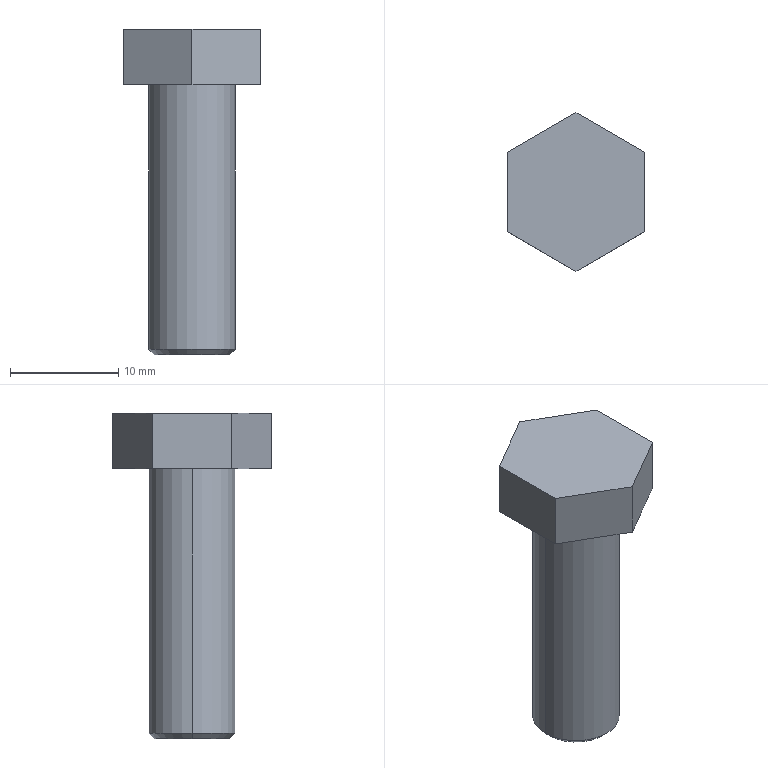Part | STEP file | Bulong M8_2.5F | 1 solid | 13 faces | box 12.73 x 14.699 x 30.15 mm | volume 1976 mm3 | plane 9 | cone 2 | cylinder 2 | commonest cylinder face diameters 8 x2
STEP:
#1=CARTESIAN_POINT('',(0.,0.,0.));
#2=DIRECTION('',(0.,0.,1.));
#3=DIRECTION('',(1.,0.,0.));
#4=AXIS2_PLACEMENT_3D('',#1,#2,#3);
#5=CARTESIAN_POINT('',(-3.5,0.,-25.));
#6=VERTEX_POINT('',#5);
#7=CARTESIAN_POINT('',(3.5,0.,-25.));
#8=VERTEX_POINT('',#7);
#9=CARTESIAN_POINT('',(0.,0.,-25.));
#10=DIRECTION('',(0.,0.,-1.));
#11=DIRECTION('',(-1.,0.,0.));
#12=AXIS2_PLACEMENT_3D('',#9,#10,#11);
#13=CIRCLE('',#12,3.5);
#14=CARTESIAN_POINT('',(0.,0.,-25.));
#15=DIRECTION('',(0.,0.,1.));
#16=DIRECTION('',(1.,0.,0.));
#17=AXIS2_PLACEMENT_3D('',#14,#15,#16);
#18=CONICAL_SURFACE('',#17,3.5,0.7854);
#19=CARTESIAN_POINT('',(3.142,0.));
#20=DIRECTION('',(-1.,0.));
#21=VECTOR('',#20,1.);
#22=LINE('',#19,#21);
#23=(GEOMETRIC_REPRESENTATION_CONTEXT(2)PARAMETRIC_REPRESENTATION_CONTEXT()REPRESENTATION_CONTEXT('',''));
#24=DEFINITIONAL_REPRESENTATION('',(#22),#23);
#25=PCURVE('',#18,#24);
#26=CARTESIAN_POINT('',(0.,0.,-25.));
#27=DIRECTION('',(0.,0.,-1.));
#28=DIRECTION('',(-1.,0.,0.));
#29=AXIS2_PLACEMENT_3D('',#26,#27,#28);
#30=PLANE('',#29);
#31=CARTESIAN_POINT('',(0.,0.));
#32=DIRECTION('',(1.,0.));
#33=AXIS2_PLACEMENT_2D('',#31,#32);
#34=CIRCLE('',#33,3.5);
#35=(GEOMETRIC_REPRESENTATION_CONTEXT(2)PARAMETRIC_REPRESENTATION_CONTEXT()REPRESENTATION_CONTEXT('',''));
#36=DEFINITIONAL_REPRESENTATION('',(#34),#35);
#37=PCURVE('',#30,#36);
#38=SURFACE_CURVE('',#13,(#25,#37),.PCURVE_S1.);
#39=EDGE_CURVE('',#6,#8,#38,.T.);
#40=ORIENTED_EDGE('',*,*,#39,.F.);
#41=CARTESIAN_POINT('',(-4.,0.,-24.5));
#42=VERTEX_POINT('',#41);
#43=CARTESIAN_POINT('',(-3.5,0.,-25.));
#44=DIRECTION('',(-0.7071,0.,0.7071));
#45=VECTOR('',#44,1.);
#46=LINE('',#43,#45);
#47=CARTESIAN_POINT('',(3.142,0.));
#48=DIRECTION('',(0.,1.));
#49=VECTOR('',#48,1.);
#50=LINE('',#47,#49);
#51=(GEOMETRIC_REPRESENTATION_CONTEXT(2)PARAMETRIC_REPRESENTATION_CONTEXT()REPRESENTATION_CONTEXT('',''));
#52=DEFINITIONAL_REPRESENTATION('',(#50),#51);
#53=PCURVE('',#18,#52);
#54=CARTESIAN_POINT('',(0.,0.,-25.));
#55=DIRECTION('',(0.,0.,1.));
#56=DIRECTION('',(1.,0.,0.));
#57=AXIS2_PLACEMENT_3D('',#54,#55,#56);
#58=CONICAL_SURFACE('',#57,3.5,0.7854);
#59=CARTESIAN_POINT('',(3.142,0.));
#60=DIRECTION('',(0.,1.));
#61=VECTOR('',#60,1.);
#62=LINE('',#59,#61);
#63=(GEOMETRIC_REPRESENTATION_CONTEXT(2)PARAMETRIC_REPRESENTATION_CONTEXT()REPRESENTATION_CONTEXT('',''));
#64=DEFINITIONAL_REPRESENTATION('',(#62),#63);
#65=PCURVE('',#58,#64);
#66=SURFACE_CURVE('',#46,(#53,#65),.PCURVE_S1.);
#67=EDGE_CURVE('',#6,#42,#66,.T.);
#68=ORIENTED_EDGE('',*,*,#67,.T.);
#69=CARTESIAN_POINT('',(4.,0.,-24.5));
#70=VERTEX_POINT('',#69);
#71=CARTESIAN_POINT('',(0.,0.,-24.5));
#72=DIRECTION('',(0.,0.,1.));
#73=DIRECTION('',(-1.,0.,0.));
#74=AXIS2_PLACEMENT_3D('',#71,#72,#73);
#75=CIRCLE('',#74,4.);
#76=CARTESIAN_POINT('',(-3.142,0.5));
#77=DIRECTION('',(1.,0.));
#78=VECTOR('',#77,1.);
#79=LINE('',#76,#78);
#80=(GEOMETRIC_REPRESENTATION_CONTEXT(2)PARAMETRIC_REPRESENTATION_CONTEXT()REPRESENTATION_CONTEXT('',''));
#81=DEFINITIONAL_REPRESENTATION('',(#79),#80);
#82=PCURVE('',#18,#81);
#83=CARTESIAN_POINT('',(0.,0.,-25.));
#84=DIRECTION('',(0.,0.,1.));
#85=DIRECTION('',(1.,0.,0.));
#86=AXIS2_PLACEMENT_3D('',#83,#84,#85);
#87=CYLINDRICAL_SURFACE('',#86,4.);
#88=CARTESIAN_POINT('',(-3.142,0.5));
#89=DIRECTION('',(1.,0.));
#90=VECTOR('',#89,1.);
#91=LINE('',#88,#90);
#92=(GEOMETRIC_REPRESENTATION_CONTEXT(2)PARAMETRIC_REPRESENTATION_CONTEXT()REPRESENTATION_CONTEXT('',''));
#93=DEFINITIONAL_REPRESENTATION('',(#91),#92);
#94=PCURVE('',#87,#93);
#95=SURFACE_CURVE('',#75,(#82,#94),.PCURVE_S1.);
#96=EDGE_CURVE('',#70,#42,#95,.T.);
#97=ORIENTED_EDGE('',*,*,#96,.F.);
#98=CARTESIAN_POINT('',(3.5,0.,-25.));
#99=DIRECTION('',(0.7071,0.,0.7071));
#100=VECTOR('',#99,1.);
#101=LINE('',#98,#100);
#102=CARTESIAN_POINT('',(0.,0.));
#103=DIRECTION('',(0.,1.));
#104=VECTOR('',#103,1.);
#105=LINE('',#102,#104);
#106=(GEOMETRIC_REPRESENTATION_CONTEXT(2)PARAMETRIC_REPRESENTATION_CONTEXT()REPRESENTATION_CONTEXT('',''));
#107=DEFINITIONAL_REPRESENTATION('',(#105),#106);
#108=PCURVE('',#18,#107);
#109=CARTESIAN_POINT('',(6.283,0.));
#110=DIRECTION('',(0.,1.));
#111=VECTOR('',#110,1.);
#112=LINE('',#109,#111);
#113=(GEOMETRIC_REPRESENTATION_CONTEXT(2)PARAMETRIC_REPRESENTATION_CONTEXT()REPRESENTATION_CONTEXT('',''));
#114=DEFINITIONAL_REPRESENTATION('',(#112),#113);
#115=PCURVE('',#58,#114);
#116=SURFACE_CURVE('',#101,(#108,#115),.PCURVE_S1.);
#117=EDGE_CURVE('',#8,#70,#116,.T.);
#118=ORIENTED_EDGE('',*,*,#117,.F.);
#119=EDGE_LOOP('',(#40,#68,#97,#118));
#120=FACE_BOUND('',#119,.T.);
#121=ADVANCED_FACE('',(#120),#18,.T.);
#122=ORIENTED_EDGE('',*,*,#96,.T.);
#123=CARTESIAN_POINT('',(-4.,0.,0.));
#124=VERTEX_POINT('',#123);
#125=CARTESIAN_POINT('',(-4.,0.,-25.));
#126=DIRECTION('',(0.,0.,1.));
#127=VECTOR('',#126,1.);
#128=LINE('',#125,#127);
#129=CARTESIAN_POINT('',(3.142,0.));
#130=DIRECTION('',(0.,1.));
#131=VECTOR('',#130,1.);
#132=LINE('',#129,#131);
#133=(GEOMETRIC_REPRESENTATION_CONTEXT(2)PARAMETRIC_REPRESENTATION_CONTEXT()REPRESENTATION_CONTEXT('',''));
#134=DEFINITIONAL_REPRESENTATION('',(#132),#133);
#135=PCURVE('',#87,#134);
#136=CARTESIAN_POINT('',(0.,0.,-25.));
#137=DIRECTION('',(0.,0.,1.));
#138=DIRECTION('',(1.,0.,0.));
#139=AXIS2_PLACEMENT_3D('',#136,#137,#138);
#140=CYLINDRICAL_SURFACE('',#139,4.);
#141=CARTESIAN_POINT('',(3.142,0.));
#142=DIRECTION('',(0.,1.));
#143=VECTOR('',#142,1.);
#144=LINE('',#141,#143);
#145=(GEOMETRIC_REPRESENTATION_CONTEXT(2)PARAMETRIC_REPRESENTATION_CONTEXT()REPRESENTATION_CONTEXT('',''));
#146=DEFINITIONAL_REPRESENTATION('',(#144),#145);
#147=PCURVE('',#140,#146);
#148=SURFACE_CURVE('',#128,(#135,#147),.PCURVE_S1.);
#149=EDGE_CURVE('',#42,#124,#148,.T.);
#150=ORIENTED_EDGE('',*,*,#149,.T.);
#151=CARTESIAN_POINT('',(4.,0.,0.));
#152=VERTEX_POINT('',#151);
#153=CARTESIAN_POINT('',(0.,0.,0.));
#154=DIRECTION('',(0.,0.,-1.));
#155=DIRECTION('',(1.,0.,0.));
#156=AXIS2_PLACEMENT_3D('',#153,#154,#155);
#157=CIRCLE('',#156,4.);
#158=CARTESIAN_POINT('',(6.283,25.));
#159=DIRECTION('',(-1.,0.));
#160=VECTOR('',#159,1.);
#161=LINE('',#158,#160);
#162=(GEOMETRIC_REPRESENTATION_CONTEXT(2)PARAMETRIC_REPRESENTATION_CONTEXT()REPRESENTATION_CONTEXT('',''));
#163=DEFINITIONAL_REPRESENTATION('',(#161),#162);
#164=PCURVE('',#87,#163);
#165=CARTESIAN_POINT('',(0.,0.,0.));
#166=DIRECTION('',(0.,0.,1.));
#167=DIRECTION('',(1.,0.,0.));
#168=AXIS2_PLACEMENT_3D('',#165,#166,#167);
#169=PLANE('',#168);
#170=CARTESIAN_POINT('',(4.,0.));
#171=CARTESIAN_POINT('',(4.,-6.928));
#172=CARTESIAN_POINT('',(-2.,-3.464));
#173=CARTESIAN_POINT('',(-8.,0.));
#174=CARTESIAN_POINT('',(-2.,3.464));
#175=CARTESIAN_POINT('',(4.,6.928));
#176=CARTESIAN_POINT('',(4.,0.));
#177=(BOUNDED_CURVE()B_SPLINE_CURVE(2,(#170,#171,#172,#173,#174,#175,#176),.UNSPECIFIED.,.T.,.F.)B_SPLINE_CURVE_WITH_KNOTS((1,2,2,2,2,1),(-2.094,0.,2.094,4.189,6.283,8.378),.UNSPECIFIED.)CURVE()GEOMETRIC_REPRESENTATION_ITEM()RATIONAL_B_SPLINE_CURVE((1.,0.5,1.,0.5,1.,0.5,1.))REPRESENTATION_ITEM(''));
#178=(GEOMETRIC_REPRESENTATION_CONTEXT(2)PARAMETRIC_REPRESENTATION_CONTEXT()REPRESENTATION_CONTEXT('',''));
#179=DEFINITIONAL_REPRESENTATION('',(#177),#178);
#180=PCURVE('',#169,#179);
#181=SURFACE_CURVE('',#157,(#164,#180),.PCURVE_S1.);
#182=EDGE_CURVE('',#124,#152,#181,.T.);
#183=ORIENTED_EDGE('',*,*,#182,.T.);
#184=CARTESIAN_POINT('',(4.,0.,-25.));
#185=DIRECTION('',(0.,0.,1.));
#186=VECTOR('',#185,1.);
#187=LINE('',#184,#186);
#188=CARTESIAN_POINT('',(0.,0.));
#189=DIRECTION('',(0.,1.));
#190=VECTOR('',#189,1.);
#191=LINE('',#188,#190);
#192=(GEOMETRIC_REPRESENTATION_CONTEXT(2)PARAMETRIC_REPRESENTATION_CONTEXT()REPRESENTATION_CONTEXT('',''));
#193=DEFINITIONAL_REPRESENTATION('',(#191),#192);
#194=PCURVE('',#87,#193);
#195=CARTESIAN_POINT('',(6.283,0.));
#196=DIRECTION('',(0.,1.));
#197=VECTOR('',#196,1.);
#198=LINE('',#195,#197);
#199=(GEOMETRIC_REPRESENTATION_CONTEXT(2)PARAMETRIC_REPRESENTATION_CONTEXT()REPRESENTATION_CONTEXT('',''));
#200=DEFINITIONAL_REPRESENTATION('',(#198),#199);
#201=PCURVE('',#140,#200);
#202=SURFACE_CURVE('',#187,(#194,#201),.PCURVE_S1.);
#203=EDGE_CURVE('',#70,#152,#202,.T.);
#204=ORIENTED_EDGE('',*,*,#203,.F.);
#205=EDGE_LOOP('',(#122,#150,#183,#204));
#206=FACE_BOUND('',#205,.T.);
#207=ADVANCED_FACE('',(#206),#87,.T.);
#208=CARTESIAN_POINT('',(6.365,3.675,0.));
#209=VERTEX_POINT('',#208);
#210=CARTESIAN_POINT('',(0.,7.35,0.));
#211=VERTEX_POINT('',#210);
#212=CARTESIAN_POINT('',(6.365,3.675,0.));
#213=DIRECTION('',(-0.866,0.5,0.));
#214=VECTOR('',#213,1.);
#215=LINE('',#212,#214);
#216=CARTESIAN_POINT('',(6.365,3.675));
#217=DIRECTION('',(-0.866,0.5));
#218=VECTOR('',#217,1.);
#219=LINE('',#216,#218);
#220=(GEOMETRIC_REPRESENTATION_CONTEXT(2)PARAMETRIC_REPRESENTATION_CONTEXT()REPRESENTATION_CONTEXT('',''));
#221=DEFINITIONAL_REPRESENTATION('',(#219),#220);
#222=PCURVE('',#169,#221);
#223=CARTESIAN_POINT('',(6.365,3.675,5.15));
#224=DIRECTION('',(-0.5,-0.866,0.));
#225=DIRECTION('',(0.866,-0.5,0.));
#226=AXIS2_PLACEMENT_3D('',#223,#224,#225);
#227=PLANE('',#226);
#228=CARTESIAN_POINT('',(0.,-5.15));
#229=DIRECTION('',(-1.,0.));
#230=VECTOR('',#229,1.);
#231=LINE('',#228,#230);
#232=(GEOMETRIC_REPRESENTATION_CONTEXT(2)PARAMETRIC_REPRESENTATION_CONTEXT()REPRESENTATION_CONTEXT('',''));
#233=DEFINITIONAL_REPRESENTATION('',(#231),#232);
#234=PCURVE('',#227,#233);
#235=SURFACE_CURVE('',#215,(#222,#234),.PCURVE_S1.);
#236=EDGE_CURVE('',#209,#211,#235,.T.);
#237=ORIENTED_EDGE('',*,*,#236,.F.);
#238=CARTESIAN_POINT('',(6.365,-3.675,0.));
#239=VERTEX_POINT('',#238);
#240=CARTESIAN_POINT('',(6.365,-3.675,0.));
#241=DIRECTION('',(0.,1.,0.));
#242=VECTOR('',#241,1.);
#243=LINE('',#240,#242);
#244=CARTESIAN_POINT('',(6.365,-3.675));
#245=DIRECTION('',(0.,1.));
#246=VECTOR('',#245,1.);
#247=LINE('',#244,#246);
#248=(GEOMETRIC_REPRESENTATION_CONTEXT(2)PARAMETRIC_REPRESENTATION_CONTEXT()REPRESENTATION_CONTEXT('',''));
#249=DEFINITIONAL_REPRESENTATION('',(#247),#248);
#250=PCURVE('',#169,#249);
#251=CARTESIAN_POINT('',(6.365,-3.675,5.15));
#252=DIRECTION('',(-1.,0.,0.));
#253=DIRECTION('',(0.,-1.,0.));
#254=AXIS2_PLACEMENT_3D('',#251,#252,#253);
#255=PLANE('',#254);
#256=CARTESIAN_POINT('',(0.,-5.15));
#257=DIRECTION('',(-1.,0.));
#258=VECTOR('',#257,1.);
#259=LINE('',#256,#258);
#260=(GEOMETRIC_REPRESENTATION_CONTEXT(2)PARAMETRIC_REPRESENTATION_CONTEXT()REPRESENTATION_CONTEXT('',''));
#261=DEFINITIONAL_REPRESENTATION('',(#259),#260);
#262=PCURVE('',#255,#261);
#263=SURFACE_CURVE('',#243,(#250,#262),.PCURVE_S1.);
#264=EDGE_CURVE('',#239,#209,#263,.T.);
#265=ORIENTED_EDGE('',*,*,#264,.F.);
#266=CARTESIAN_POINT('',(0.,-7.35,0.));
#267=VERTEX_POINT('',#266);
#268=CARTESIAN_POINT('',(0.,-7.35,0.));
#269=DIRECTION('',(0.866,0.5,0.));
#270=VECTOR('',#269,1.);
#271=LINE('',#268,#270);
#272=CARTESIAN_POINT('',(0.,-7.35));
#273=DIRECTION('',(0.866,0.5));
#274=VECTOR('',#273,1.);
#275=LINE('',#272,#274);
#276=(GEOMETRIC_REPRESENTATION_CONTEXT(2)PARAMETRIC_REPRESENTATION_CONTEXT()REPRESENTATION_CONTEXT('',''));
#277=DEFINITIONAL_REPRESENTATION('',(#275),#276);
#278=PCURVE('',#169,#277);
#279=CARTESIAN_POINT('',(0.,-7.35,5.15));
#280=DIRECTION('',(-0.5,0.866,0.));
#281=DIRECTION('',(-0.866,-0.5,0.));
#282=AXIS2_PLACEMENT_3D('',#279,#280,#281);
#283=PLANE('',#282);
#284=CARTESIAN_POINT('',(0.,-5.15));
#285=DIRECTION('',(-1.,0.));
#286=VECTOR('',#285,1.);
#287=LINE('',#284,#286);
#288=(GEOMETRIC_REPRESENTATION_CONTEXT(2)PARAMETRIC_REPRESENTATION_CONTEXT()REPRESENTATION_CONTEXT('',''));
#289=DEFINITIONAL_REPRESENTATION('',(#287),#288);
#290=PCURVE('',#283,#289);
#291=SURFACE_CURVE('',#271,(#278,#290),.PCURVE_S1.);
#292=EDGE_CURVE('',#267,#239,#291,.T.);
#293=ORIENTED_EDGE('',*,*,#292,.F.);
#294=CARTESIAN_POINT('',(-6.365,-3.675,0.));
#295=VERTEX_POINT('',#294);
#296=CARTESIAN_POINT('',(-6.365,-3.675,0.));
#297=DIRECTION('',(0.866,-0.5,0.));
#298=VECTOR('',#297,1.);
#299=LINE('',#296,#298);
#300=CARTESIAN_POINT('',(-6.365,-3.675));
#301=DIRECTION('',(0.866,-0.5));
#302=VECTOR('',#301,1.);
#303=LINE('',#300,#302);
#304=(GEOMETRIC_REPRESENTATION_CONTEXT(2)PARAMETRIC_REPRESENTATION_CONTEXT()REPRESENTATION_CONTEXT('',''));
#305=DEFINITIONAL_REPRESENTATION('',(#303),#304);
#306=PCURVE('',#169,#305);
#307=CARTESIAN_POINT('',(-6.365,-3.675,5.15));
#308=DIRECTION('',(0.5,0.866,0.));
#309=DIRECTION('',(-0.866,0.5,0.));
#310=AXIS2_PLACEMENT_3D('',#307,#308,#309);
#311=PLANE('',#310);
#312=CARTESIAN_POINT('',(0.,-5.15));
#313=DIRECTION('',(-1.,0.));
#314=VECTOR('',#313,1.);
#315=LINE('',#312,#314);
#316=(GEOMETRIC_REPRESENTATION_CONTEXT(2)PARAMETRIC_REPRESENTATION_CONTEXT()REPRESENTATION_CONTEXT('',''));
#317=DEFINITIONAL_REPRESENTATION('',(#315),#316);
#318=PCURVE('',#311,#317);
#319=SURFACE_CURVE('',#299,(#306,#318),.PCURVE_S1.);
#320=EDGE_CURVE('',#295,#267,#319,.T.);
#321=ORIENTED_EDGE('',*,*,#320,.F.);
#322=CARTESIAN_POINT('',(-6.365,3.675,0.));
#323=VERTEX_POINT('',#322);
#324=CARTESIAN_POINT('',(-6.365,3.675,0.));
#325=DIRECTION('',(0.,-1.,0.));
#326=VECTOR('',#325,1.);
#327=LINE('',#324,#326);
#328=CARTESIAN_POINT('',(-6.365,3.675));
#329=DIRECTION('',(0.,-1.));
#330=VECTOR('',#329,1.);
#331=LINE('',#328,#330);
#332=(GEOMETRIC_REPRESENTATION_CONTEXT(2)PARAMETRIC_REPRESENTATION_CONTEXT()REPRESENTATION_CONTEXT('',''));
#333=DEFINITIONAL_REPRESENTATION('',(#331),#332);
#334=PCURVE('',#169,#333);
#335=CARTESIAN_POINT('',(-6.365,3.675,5.15));
#336=DIRECTION('',(1.,0.,0.));
#337=DIRECTION('',(0.,0.,-1.));
#338=AXIS2_PLACEMENT_3D('',#335,#336,#337);
#339=PLANE('',#338);
#340=CARTESIAN_POINT('',(5.15,0.));
#341=DIRECTION('',(0.,-1.));
#342=VECTOR('',#341,1.);
#343=LINE('',#340,#342);
#344=(GEOMETRIC_REPRESENTATION_CONTEXT(2)PARAMETRIC_REPRESENTATION_CONTEXT()REPRESENTATION_CONTEXT('',''));
#345=DEFINITIONAL_REPRESENTATION('',(#343),#344);
#346=PCURVE('',#339,#345);
#347=SURFACE_CURVE('',#327,(#334,#346),.PCURVE_S1.);
#348=EDGE_CURVE('',#323,#295,#347,.T.);
#349=ORIENTED_EDGE('',*,*,#348,.F.);
#350=CARTESIAN_POINT('',(0.,7.35,0.));
#351=DIRECTION('',(-0.866,-0.5,0.));
#352=VECTOR('',#351,1.);
#353=LINE('',#350,#352);
#354=CARTESIAN_POINT('',(0.,7.35));
#355=DIRECTION('',(-0.866,-0.5));
#356=VECTOR('',#355,1.);
#357=LINE('',#354,#356);
#358=(GEOMETRIC_REPRESENTATION_CONTEXT(2)PARAMETRIC_REPRESENTATION_CONTEXT()REPRESENTATION_CONTEXT('',''));
#359=DEFINITIONAL_REPRESENTATION('',(#357),#358);
#360=PCURVE('',#169,#359);
#361=CARTESIAN_POINT('',(0.,7.35,5.15));
#362=DIRECTION('',(0.5,-0.866,0.));
#363=DIRECTION('',(0.866,0.5,0.));
#364=AXIS2_PLACEMENT_3D('',#361,#362,#363);
#365=PLANE('',#364);
#366=CARTESIAN_POINT('',(0.,-5.15));
#367=DIRECTION('',(-1.,0.));
#368=VECTOR('',#367,1.);
#369=LINE('',#366,#368);
#370=(GEOMETRIC_REPRESENTATION_CONTEXT(2)PARAMETRIC_REPRESENTATION_CONTEXT()REPRESENTATION_CONTEXT('',''));
#371=DEFINITIONAL_REPRESENTATION('',(#369),#370);
#372=PCURVE('',#365,#371);
#373=SURFACE_CURVE('',#353,(#360,#372),.PCURVE_S1.);
#374=EDGE_CURVE('',#211,#323,#373,.T.);
#375=ORIENTED_EDGE('',*,*,#374,.F.);
#376=EDGE_LOOP('',(#237,#265,#293,#321,#349,#375));
#377=FACE_BOUND('',#376,.T.);
#378=CARTESIAN_POINT('',(0.,0.,0.));
#379=DIRECTION('',(0.,0.,-1.));
#380=DIRECTION('',(1.,0.,0.));
#381=AXIS2_PLACEMENT_3D('',#378,#379,#380);
#382=CIRCLE('',#381,4.);
#383=CARTESIAN_POINT('',(4.,0.));
#384=CARTESIAN_POINT('',(4.,-6.928));
#385=CARTESIAN_POINT('',(-2.,-3.464));
#386=CARTESIAN_POINT('',(-8.,0.));
#387=CARTESIAN_POINT('',(-2.,3.464));
#388=CARTESIAN_POINT('',(4.,6.928));
#389=CARTESIAN_POINT('',(4.,0.));
#390=(BOUNDED_CURVE()B_SPLINE_CURVE(2,(#383,#384,#385,#386,#387,#388,#389),.UNSPECIFIED.,.T.,.F.)B_SPLINE_CURVE_WITH_KNOTS((1,2,2,2,2,1),(-2.094,0.,2.094,4.189,6.283,8.378),.UNSPECIFIED.)CURVE()GEOMETRIC_REPRESENTATION_ITEM()RATIONAL_B_SPLINE_CURVE((1.,0.5,1.,0.5,1.,0.5,1.))REPRESENTATION_ITEM(''));
#391=(GEOMETRIC_REPRESENTATION_CONTEXT(2)PARAMETRIC_REPRESENTATION_CONTEXT()REPRESENTATION_CONTEXT('',''));
#392=DEFINITIONAL_REPRESENTATION('',(#390),#391);
#393=PCURVE('',#169,#392);
#394=CARTESIAN_POINT('',(6.283,25.));
#395=DIRECTION('',(-1.,0.));
#396=VECTOR('',#395,1.);
#397=LINE('',#394,#396);
#398=(GEOMETRIC_REPRESENTATION_CONTEXT(2)PARAMETRIC_REPRESENTATION_CONTEXT()REPRESENTATION_CONTEXT('',''));
#399=DEFINITIONAL_REPRESENTATION('',(#397),#398);
#400=PCURVE('',#140,#399);
#401=SURFACE_CURVE('',#382,(#393,#400),.PCURVE_S1.);
#402=EDGE_CURVE('',#152,#124,#401,.T.);
#403=ORIENTED_EDGE('',*,*,#402,.F.);
#404=ORIENTED_EDGE('',*,*,#182,.F.);
#405=EDGE_LOOP('',(#403,#404));
#406=FACE_BOUND('',#405,.T.);
#407=ADVANCED_FACE('',(#377,#406),#169,.F.);
#408=ORIENTED_EDGE('',*,*,#236,.T.);
#409=CARTESIAN_POINT('',(0.,7.35,5.15));
#410=VERTEX_POINT('',#409);
#411=CARTESIAN_POINT('',(0.,7.35,5.15));
#412=DIRECTION('',(0.,0.,-1.));
#413=VECTOR('',#412,1.);
#414=LINE('',#411,#413);
#415=CARTESIAN_POINT('',(-7.35,0.));
#416=DIRECTION('',(0.,-1.));
#417=VECTOR('',#416,1.);
#418=LINE('',#415,#417);
#419=(GEOMETRIC_REPRESENTATION_CONTEXT(2)PARAMETRIC_REPRESENTATION_CONTEXT()REPRESENTATION_CONTEXT('',''));
#420=DEFINITIONAL_REPRESENTATION('',(#418),#419);
#421=PCURVE('',#227,#420);
#422=CARTESIAN_POINT('',(0.,0.));
#423=DIRECTION('',(0.,-1.));
#424=VECTOR('',#423,1.);
#425=LINE('',#422,#424);
#426=(GEOMETRIC_REPRESENTATION_CONTEXT(2)PARAMETRIC_REPRESENTATION_CONTEXT()REPRESENTATION_CONTEXT('',''));
#427=DEFINITIONAL_REPRESENTATION('',(#425),#426);
#428=PCURVE('',#365,#427);
#429=SURFACE_CURVE('',#414,(#421,#428),.PCURVE_S1.);
#430=EDGE_CURVE('',#410,#211,#429,.T.);
#431=ORIENTED_EDGE('',*,*,#430,.F.);
#432=CARTESIAN_POINT('',(6.365,3.675,5.15));
#433=VERTEX_POINT('',#432);
#434=CARTESIAN_POINT('',(6.365,3.675,5.15));
#435=DIRECTION('',(-0.866,0.5,0.));
#436=VECTOR('',#435,1.);
#437=LINE('',#434,#436);
#438=CARTESIAN_POINT('',(0.,0.));
#439=DIRECTION('',(-1.,0.));
#440=VECTOR('',#439,1.);
#441=LINE('',#438,#440);
#442=(GEOMETRIC_REPRESENTATION_CONTEXT(2)PARAMETRIC_REPRESENTATION_CONTEXT()REPRESENTATION_CONTEXT('',''));
#443=DEFINITIONAL_REPRESENTATION('',(#441),#442);
#444=PCURVE('',#227,#443);
#445=CARTESIAN_POINT('',(0.,0.,5.15));
#446=DIRECTION('',(0.,0.,1.));
#447=DIRECTION('',(1.,0.,0.));
#448=AXIS2_PLACEMENT_3D('',#445,#446,#447);
#449=PLANE('',#448);
#450=CARTESIAN_POINT('',(6.365,3.675));
#451=DIRECTION('',(-0.866,0.5));
#452=VECTOR('',#451,1.);
#453=LINE('',#450,#452);
#454=(GEOMETRIC_REPRESENTATION_CONTEXT(2)PARAMETRIC_REPRESENTATION_CONTEXT()REPRESENTATION_CONTEXT('',''));
#455=DEFINITIONAL_REPRESENTATION('',(#453),#454);
#456=PCURVE('',#449,#455);
#457=SURFACE_CURVE('',#437,(#444,#456),.PCURVE_S1.);
#458=EDGE_CURVE('',#433,#410,#457,.T.);
#459=ORIENTED_EDGE('',*,*,#458,.F.);
#460=CARTESIAN_POINT('',(6.365,3.675,5.15));
#461=DIRECTION('',(0.,0.,-1.));
#462=VECTOR('',#461,1.);
#463=LINE('',#460,#462);
#464=CARTESIAN_POINT('',(0.,0.));
#465=DIRECTION('',(0.,-1.));
#466=VECTOR('',#465,1.);
#467=LINE('',#464,#466);
#468=(GEOMETRIC_REPRESENTATION_CONTEXT(2)PARAMETRIC_REPRESENTATION_CONTEXT()REPRESENTATION_CONTEXT('',''));
#469=DEFINITIONAL_REPRESENTATION('',(#467),#468);
#470=PCURVE('',#227,#469);
#471=CARTESIAN_POINT('',(-7.35,0.));
#472=DIRECTION('',(0.,-1.));
#473=VECTOR('',#472,1.);
#474=LINE('',#471,#473);
#475=(GEOMETRIC_REPRESENTATION_CONTEXT(2)PARAMETRIC_REPRESENTATION_CONTEXT()REPRESENTATION_CONTEXT('',''));
#476=DEFINITIONAL_REPRESENTATION('',(#474),#475);
#477=PCURVE('',#255,#476);
#478=SURFACE_CURVE('',#463,(#470,#477),.PCURVE_S1.);
#479=EDGE_CURVE('',#433,#209,#478,.T.);
#480=ORIENTED_EDGE('',*,*,#479,.T.);
#481=EDGE_LOOP('',(#408,#431,#459,#480));
#482=FACE_BOUND('',#481,.T.);
#483=ADVANCED_FACE('',(#482),#227,.F.);
#484=ORIENTED_EDGE('',*,*,#374,.T.);
#485=CARTESIAN_POINT('',(-6.365,3.675,5.15));
#486=VERTEX_POINT('',#485);
#487=CARTESIAN_POINT('',(-6.365,3.675,5.15));
#488=DIRECTION('',(0.,0.,-1.));
#489=VECTOR('',#488,1.);
#490=LINE('',#487,#489);
#491=CARTESIAN_POINT('',(-7.35,0.));
#492=DIRECTION('',(0.,-1.));
#493=VECTOR('',#492,1.);
#494=LINE('',#491,#493);
#495=(GEOMETRIC_REPRESENTATION_CONTEXT(2)PARAMETRIC_REPRESENTATION_CONTEXT()REPRESENTATION_CONTEXT('',''));
#496=DEFINITIONAL_REPRESENTATION('',(#494),#495);
#497=PCURVE('',#365,#496);
#498=CARTESIAN_POINT('',(0.,0.));
#499=DIRECTION('',(1.,0.));
#500=VECTOR('',#499,1.);
#501=LINE('',#498,#500);
#502=(GEOMETRIC_REPRESENTATION_CONTEXT(2)PARAMETRIC_REPRESENTATION_CONTEXT()REPRESENTATION_CONTEXT('',''));
#503=DEFINITIONAL_REPRESENTATION('',(#501),#502);
#504=PCURVE('',#339,#503);
#505=SURFACE_CURVE('',#490,(#497,#504),.PCURVE_S1.);
#506=EDGE_CURVE('',#486,#323,#505,.T.);
#507=ORIENTED_EDGE('',*,*,#506,.F.);
#508=CARTESIAN_POINT('',(0.,7.35,5.15));
#509=DIRECTION('',(-0.866,-0.5,0.));
#510=VECTOR('',#509,1.);
#511=LINE('',#508,#510);
#512=CARTESIAN_POINT('',(0.,0.));
#513=DIRECTION('',(-1.,0.));
#514=VECTOR('',#513,1.);
#515=LINE('',#512,#514);
#516=(GEOMETRIC_REPRESENTATION_CONTEXT(2)PARAMETRIC_REPRESENTATION_CONTEXT()REPRESENTATION_CONTEXT('',''));
#517=DEFINITIONAL_REPRESENTATION('',(#515),#516);
#518=PCURVE('',#365,#517);
#519=CARTESIAN_POINT('',(0.,7.35));
#520=DIRECTION('',(-0.866,-0.5));
#521=VECTOR('',#520,1.);
#522=LINE('',#519,#521);
#523=(GEOMETRIC_REPRESENTATION_CONTEXT(2)PARAMETRIC_REPRESENTATION_CONTEXT()REPRESENTATION_CONTEXT('',''));
#524=DEFINITIONAL_REPRESENTATION('',(#522),#523);
#525=PCURVE('',#449,#524);
#526=SURFACE_CURVE('',#511,(#518,#525),.PCURVE_S1.);
#527=EDGE_CURVE('',#410,#486,#526,.T.);
#528=ORIENTED_EDGE('',*,*,#527,.F.);
#529=ORIENTED_EDGE('',*,*,#430,.T.);
#530=EDGE_LOOP('',(#484,#507,#528,#529));
#531=FACE_BOUND('',#530,.T.);
#532=ADVANCED_FACE('',(#531),#365,.F.);
#533=ORIENTED_EDGE('',*,*,#348,.T.);
#534=CARTESIAN_POINT('',(-6.365,-3.675,5.15));
#535=VERTEX_POINT('',#534);
#536=CARTESIAN_POINT('',(-6.365,-3.675,5.15));
#537=DIRECTION('',(0.,0.,-1.));
#538=VECTOR('',#537,1.);
#539=LINE('',#536,#538);
#540=CARTESIAN_POINT('',(0.,-7.35));
#541=DIRECTION('',(1.,0.));
#542=VECTOR('',#541,1.);
#543=LINE('',#540,#542);
#544=(GEOMETRIC_REPRESENTATION_CONTEXT(2)PARAMETRIC_REPRESENTATION_CONTEXT()REPRESENTATION_CONTEXT('',''));
#545=DEFINITIONAL_REPRESENTATION('',(#543),#544);
#546=PCURVE('',#339,#545);
#547=CARTESIAN_POINT('',(0.,0.));
#548=DIRECTION('',(0.,-1.));
#549=VECTOR('',#548,1.);
#550=LINE('',#547,#549);
#551=(GEOMETRIC_REPRESENTATION_CONTEXT(2)PARAMETRIC_REPRESENTATION_CONTEXT()REPRESENTATION_CONTEXT('',''));
#552=DEFINITIONAL_REPRESENTATION('',(#550),#551);
#553=PCURVE('',#311,#552);
#554=SURFACE_CURVE('',#539,(#546,#553),.PCURVE_S1.);
#555=EDGE_CURVE('',#535,#295,#554,.T.);
#556=ORIENTED_EDGE('',*,*,#555,.F.);
#557=CARTESIAN_POINT('',(-6.365,3.675,5.15));
#558=DIRECTION('',(0.,-1.,0.));
#559=VECTOR('',#558,1.);
#560=LINE('',#557,#559);
#561=CARTESIAN_POINT('',(0.,0.));
#562=DIRECTION('',(0.,-1.));
#563=VECTOR('',#562,1.);
#564=LINE('',#561,#563);
#565=(GEOMETRIC_REPRESENTATION_CONTEXT(2)PARAMETRIC_REPRESENTATION_CONTEXT()REPRESENTATION_CONTEXT('',''));
#566=DEFINITIONAL_REPRESENTATION('',(#564),#565);
#567=PCURVE('',#339,#566);
#568=CARTESIAN_POINT('',(-6.365,3.675));
#569=DIRECTION('',(0.,-1.));
#570=VECTOR('',#569,1.);
#571=LINE('',#568,#570);
#572=(GEOMETRIC_REPRESENTATION_CONTEXT(2)PARAMETRIC_REPRESENTATION_CONTEXT()REPRESENTATION_CONTEXT('',''));
#573=DEFINITIONAL_REPRESENTATION('',(#571),#572);
#574=PCURVE('',#449,#573);
#575=SURFACE_CURVE('',#560,(#567,#574),.PCURVE_S1.);
#576=EDGE_CURVE('',#486,#535,#575,.T.);
#577=ORIENTED_EDGE('',*,*,#576,.F.);
#578=ORIENTED_EDGE('',*,*,#506,.T.);
#579=EDGE_LOOP('',(#533,#556,#577,#578));
#580=FACE_BOUND('',#579,.T.);
#581=ADVANCED_FACE('',(#580),#339,.F.);
#582=ORIENTED_EDGE('',*,*,#320,.T.);
#583=CARTESIAN_POINT('',(0.,-7.35,5.15));
#584=VERTEX_POINT('',#583);
#585=CARTESIAN_POINT('',(0.,-7.35,5.15));
#586=DIRECTION('',(0.,0.,-1.));
#587=VECTOR('',#586,1.);
#588=LINE('',#585,#587);
#589=CARTESIAN_POINT('',(-7.35,0.));
#590=DIRECTION('',(0.,-1.));
#591=VECTOR('',#590,1.);
#592=LINE('',#589,#591);
#593=(GEOMETRIC_REPRESENTATION_CONTEXT(2)PARAMETRIC_REPRESENTATION_CONTEXT()REPRESENTATION_CONTEXT('',''));
#594=DEFINITIONAL_REPRESENTATION('',(#592),#593);
#595=PCURVE('',#311,#594);
#596=CARTESIAN_POINT('',(0.,0.));
#597=DIRECTION('',(0.,-1.));
#598=VECTOR('',#597,1.);
#599=LINE('',#596,#598);
#600=(GEOMETRIC_REPRESENTATION_CONTEXT(2)PARAMETRIC_REPRESENTATION_CONTEXT()REPRESENTATION_CONTEXT('',''));
#601=DEFINITIONAL_REPRESENTATION('',(#599),#600);
#602=PCURVE('',#283,#601);
#603=SURFACE_CURVE('',#588,(#595,#602),.PCURVE_S1.);
#604=EDGE_CURVE('',#584,#267,#603,.T.);
#605=ORIENTED_EDGE('',*,*,#604,.F.);
#606=CARTESIAN_POINT('',(-6.365,-3.675,5.15));
#607=DIRECTION('',(0.866,-0.5,0.));
#608=VECTOR('',#607,1.);
#609=LINE('',#606,#608);
#610=CARTESIAN_POINT('',(0.,0.));
#611=DIRECTION('',(-1.,0.));
#612=VECTOR('',#611,1.);
#613=LINE('',#610,#612);
#614=(GEOMETRIC_REPRESENTATION_CONTEXT(2)PARAMETRIC_REPRESENTATION_CONTEXT()REPRESENTATION_CONTEXT('',''));
#615=DEFINITIONAL_REPRESENTATION('',(#613),#614);
#616=PCURVE('',#311,#615);
#617=CARTESIAN_POINT('',(-6.365,-3.675));
#618=DIRECTION('',(0.866,-0.5));
#619=VECTOR('',#618,1.);
#620=LINE('',#617,#619);
#621=(GEOMETRIC_REPRESENTATION_CONTEXT(2)PARAMETRIC_REPRESENTATION_CONTEXT()REPRESENTATION_CONTEXT('',''));
#622=DEFINITIONAL_REPRESENTATION('',(#620),#621);
#623=PCURVE('',#449,#622);
#624=SURFACE_CURVE('',#609,(#616,#623),.PCURVE_S1.);
#625=EDGE_CURVE('',#535,#584,#624,.T.);
#626=ORIENTED_EDGE('',*,*,#625,.F.);
#627=ORIENTED_EDGE('',*,*,#555,.T.);
#628=EDGE_LOOP('',(#582,#605,#626,#627));
#629=FACE_BOUND('',#628,.T.);
#630=ADVANCED_FACE('',(#629),#311,.F.);
#631=ORIENTED_EDGE('',*,*,#292,.T.);
#632=CARTESIAN_POINT('',(6.365,-3.675,5.15));
#633=VERTEX_POINT('',#632);
#634=CARTESIAN_POINT('',(6.365,-3.675,5.15));
#635=DIRECTION('',(0.,0.,-1.));
#636=VECTOR('',#635,1.);
#637=LINE('',#634,#636);
#638=CARTESIAN_POINT('',(-7.35,0.));
#639=DIRECTION('',(0.,-1.));
#640=VECTOR('',#639,1.);
#641=LINE('',#638,#640);
#642=(GEOMETRIC_REPRESENTATION_CONTEXT(2)PARAMETRIC_REPRESENTATION_CONTEXT()REPRESENTATION_CONTEXT('',''));
#643=DEFINITIONAL_REPRESENTATION('',(#641),#642);
#644=PCURVE('',#283,#643);
#645=CARTESIAN_POINT('',(0.,0.));
#646=DIRECTION('',(0.,-1.));
#647=VECTOR('',#646,1.);
#648=LINE('',#645,#647);
#649=(GEOMETRIC_REPRESENTATION_CONTEXT(2)PARAMETRIC_REPRESENTATION_CONTEXT()REPRESENTATION_CONTEXT('',''));
#650=DEFINITIONAL_REPRESENTATION('',(#648),#649);
#651=PCURVE('',#255,#650);
#652=SURFACE_CURVE('',#637,(#644,#651),.PCURVE_S1.);
#653=EDGE_CURVE('',#633,#239,#652,.T.);
#654=ORIENTED_EDGE('',*,*,#653,.F.);
#655=CARTESIAN_POINT('',(0.,-7.35,5.15));
#656=DIRECTION('',(0.866,0.5,0.));
#657=VECTOR('',#656,1.);
#658=LINE('',#655,#657);
#659=CARTESIAN_POINT('',(0.,0.));
#660=DIRECTION('',(-1.,0.));
#661=VECTOR('',#660,1.);
#662=LINE('',#659,#661);
#663=(GEOMETRIC_REPRESENTATION_CONTEXT(2)PARAMETRIC_REPRESENTATION_CONTEXT()REPRESENTATION_CONTEXT('',''));
#664=DEFINITIONAL_REPRESENTATION('',(#662),#663);
#665=PCURVE('',#283,#664);
#666=CARTESIAN_POINT('',(0.,-7.35));
#667=DIRECTION('',(0.866,0.5));
#668=VECTOR('',#667,1.);
#669=LINE('',#666,#668);
#670=(GEOMETRIC_REPRESENTATION_CONTEXT(2)PARAMETRIC_REPRESENTATION_CONTEXT()REPRESENTATION_CONTEXT('',''));
#671=DEFINITIONAL_REPRESENTATION('',(#669),#670);
#672=PCURVE('',#449,#671);
#673=SURFACE_CURVE('',#658,(#665,#672),.PCURVE_S1.);
#674=EDGE_CURVE('',#584,#633,#673,.T.);
#675=ORIENTED_EDGE('',*,*,#674,.F.);
#676=ORIENTED_EDGE('',*,*,#604,.T.);
#677=EDGE_LOOP('',(#631,#654,#675,#676));
#678=FACE_BOUND('',#677,.T.);
#679=ADVANCED_FACE('',(#678),#283,.F.);
#680=ORIENTED_EDGE('',*,*,#264,.T.);
#681=ORIENTED_EDGE('',*,*,#479,.F.);
#682=CARTESIAN_POINT('',(6.365,-3.675,5.15));
#683=DIRECTION('',(0.,1.,0.));
#684=VECTOR('',#683,1.);
#685=LINE('',#682,#684);
#686=CARTESIAN_POINT('',(0.,0.));
#687=DIRECTION('',(-1.,0.));
#688=VECTOR('',#687,1.);
#689=LINE('',#686,#688);
#690=(GEOMETRIC_REPRESENTATION_CONTEXT(2)PARAMETRIC_REPRESENTATION_CONTEXT()REPRESENTATION_CONTEXT('',''));
#691=DEFINITIONAL_REPRESENTATION('',(#689),#690);
#692=PCURVE('',#255,#691);
#693=CARTESIAN_POINT('',(6.365,-3.675));
#694=DIRECTION('',(0.,1.));
#695=VECTOR('',#694,1.);
#696=LINE('',#693,#695);
#697=(GEOMETRIC_REPRESENTATION_CONTEXT(2)PARAMETRIC_REPRESENTATION_CONTEXT()REPRESENTATION_CONTEXT('',''));
#698=DEFINITIONAL_REPRESENTATION('',(#696),#697);
#699=PCURVE('',#449,#698);
#700=SURFACE_CURVE('',#685,(#692,#699),.PCURVE_S1.);
#701=EDGE_CURVE('',#633,#433,#700,.T.);
#702=ORIENTED_EDGE('',*,*,#701,.F.);
#703=ORIENTED_EDGE('',*,*,#653,.T.);
#704=EDGE_LOOP('',(#680,#681,#702,#703));
#705=FACE_BOUND('',#704,.T.);
#706=ADVANCED_FACE('',(#705),#255,.F.);
#707=ORIENTED_EDGE('',*,*,#458,.T.);
#708=ORIENTED_EDGE('',*,*,#527,.T.);
#709=ORIENTED_EDGE('',*,*,#576,.T.);
#710=ORIENTED_EDGE('',*,*,#625,.T.);
#711=ORIENTED_EDGE('',*,*,#674,.T.);
#712=ORIENTED_EDGE('',*,*,#701,.T.);
#713=EDGE_LOOP('',(#707,#708,#709,#710,#711,#712));
#714=FACE_BOUND('',#713,.T.);
#715=ADVANCED_FACE('',(#714),#449,.T.);
#716=ORIENTED_EDGE('',*,*,#149,.F.);
#717=CARTESIAN_POINT('',(0.,0.,-24.5));
#718=DIRECTION('',(0.,0.,1.));
#719=DIRECTION('',(-1.,0.,0.));
#720=AXIS2_PLACEMENT_3D('',#717,#718,#719);
#721=CIRCLE('',#720,4.);
#722=CARTESIAN_POINT('',(3.142,0.5));
#723=DIRECTION('',(1.,0.));
#724=VECTOR('',#723,1.);
#725=LINE('',#722,#724);
#726=(GEOMETRIC_REPRESENTATION_CONTEXT(2)PARAMETRIC_REPRESENTATION_CONTEXT()REPRESENTATION_CONTEXT('',''));
#727=DEFINITIONAL_REPRESENTATION('',(#725),#726);
#728=PCURVE('',#140,#727);
#729=CARTESIAN_POINT('',(3.142,0.5));
#730=DIRECTION('',(1.,0.));
#731=VECTOR('',#730,1.);
#732=LINE('',#729,#731);
#733=(GEOMETRIC_REPRESENTATION_CONTEXT(2)PARAMETRIC_REPRESENTATION_CONTEXT()REPRESENTATION_CONTEXT('',''));
#734=DEFINITIONAL_REPRESENTATION('',(#732),#733);
#735=PCURVE('',#58,#734);
#736=SURFACE_CURVE('',#721,(#728,#735),.PCURVE_S1.);
#737=EDGE_CURVE('',#42,#70,#736,.T.);
#738=ORIENTED_EDGE('',*,*,#737,.T.);
#739=ORIENTED_EDGE('',*,*,#203,.T.);
#740=ORIENTED_EDGE('',*,*,#402,.T.);
#741=EDGE_LOOP('',(#716,#738,#739,#740));
#742=FACE_BOUND('',#741,.T.);
#743=ADVANCED_FACE('',(#742),#140,.T.);
#744=CARTESIAN_POINT('',(0.,0.,-25.));
#745=DIRECTION('',(0.,0.,-1.));
#746=DIRECTION('',(-1.,0.,0.));
#747=AXIS2_PLACEMENT_3D('',#744,#745,#746);
#748=CIRCLE('',#747,3.5);
#749=CARTESIAN_POINT('',(0.,0.));
#750=DIRECTION('',(1.,0.));
#751=AXIS2_PLACEMENT_2D('',#749,#750);
#752=CIRCLE('',#751,3.5);
#753=(GEOMETRIC_REPRESENTATION_CONTEXT(2)PARAMETRIC_REPRESENTATION_CONTEXT()REPRESENTATION_CONTEXT('',''));
#754=DEFINITIONAL_REPRESENTATION('',(#752),#753);
#755=PCURVE('',#30,#754);
#756=CARTESIAN_POINT('',(9.425,0.));
#757=DIRECTION('',(-1.,0.));
#758=VECTOR('',#757,1.);
#759=LINE('',#756,#758);
#760=(GEOMETRIC_REPRESENTATION_CONTEXT(2)PARAMETRIC_REPRESENTATION_CONTEXT()REPRESENTATION_CONTEXT('',''));
#761=DEFINITIONAL_REPRESENTATION('',(#759),#760);
#762=PCURVE('',#58,#761);
#763=SURFACE_CURVE('',#748,(#755,#762),.PCURVE_S1.);
#764=EDGE_CURVE('',#8,#6,#763,.T.);
#765=ORIENTED_EDGE('',*,*,#764,.T.);
#766=ORIENTED_EDGE('',*,*,#39,.T.);
#767=EDGE_LOOP('',(#765,#766));
#768=FACE_BOUND('',#767,.T.);
#769=ADVANCED_FACE('',(#768),#30,.T.);
#770=ORIENTED_EDGE('',*,*,#67,.F.);
#771=ORIENTED_EDGE('',*,*,#764,.F.);
#772=ORIENTED_EDGE('',*,*,#117,.T.);
#773=ORIENTED_EDGE('',*,*,#737,.F.);
#774=EDGE_LOOP('',(#770,#771,#772,#773));
#775=FACE_BOUND('',#774,.T.);
#776=ADVANCED_FACE('',(#775),#58,.T.);
#777=CLOSED_SHELL('',(#121,#207,#407,#483,#532,#581,#630,#679,#706,#715,#743,#769,#776));
#778=MANIFOLD_SOLID_BREP('',#777);
#779=(LENGTH_UNIT()NAMED_UNIT(*)SI_UNIT(.MILLI.,.METRE.));
#780=UNCERTAINTY_MEASURE_WITH_UNIT(LENGTH_MEASURE(0.0000001),#779,'','');
#781=(NAMED_UNIT(*)PLANE_ANGLE_UNIT()SI_UNIT($,.RADIAN.));
#782=(NAMED_UNIT(*)SI_UNIT($,.STERADIAN.)SOLID_ANGLE_UNIT());
#783=(GEOMETRIC_REPRESENTATION_CONTEXT(3)GLOBAL_UNCERTAINTY_ASSIGNED_CONTEXT((#780))GLOBAL_UNIT_ASSIGNED_CONTEXT((#779,#781,#782))REPRESENTATION_CONTEXT('',''));
#784=ADVANCED_BREP_SHAPE_REPRESENTATION('',(#4,#778),#783);